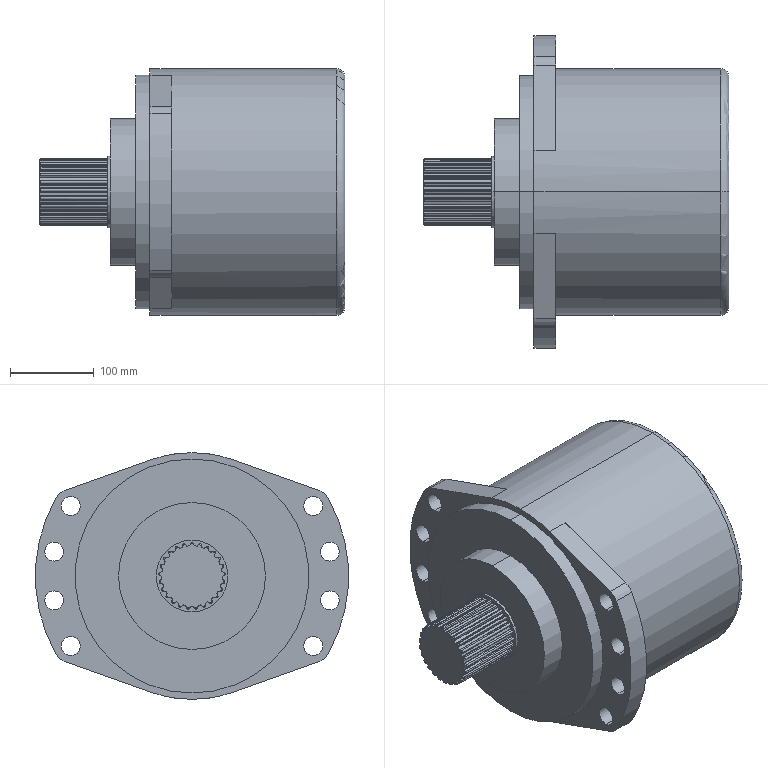Part | SolidWorks | features ICE 2, RevCut 1, Revolution 1 | 1 solid | 228 faces | box 366 x 375 x 295 mm | volume 18545806 mm3 | cylinder 189 | cone 25 | plane 12 | torus 2 | commonest cylinder face diameters 33.952 x50 38.829 x50 3.36 x34 72.3 x25 22.5 x16 40 x4